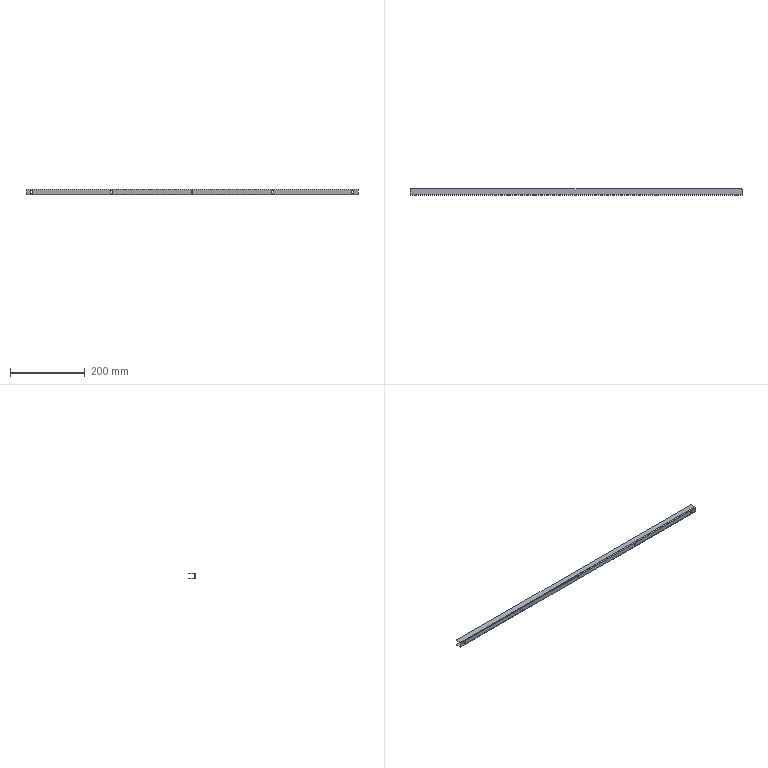Part | NX | features BREP 1 | 1 solid | 51 faces | box 890 x 17 x 15 mm | volume 40494 mm3 | plane 28 | cylinder 23 | commonest cylinder face diameters 4.8 x15 4 x6 2 x2
STEP:
#1=CARTESIAN_POINT('',(445.,14.,7.5));
#2=VERTEX_POINT('',#1);
#3=CARTESIAN_POINT('',(443.,16.,7.5));
#4=VERTEX_POINT('',#3);
#5=CARTESIAN_POINT('',(443.,14.,7.5));
#6=DIRECTION('',(0.,0.,1.));
#7=DIRECTION('',(-1.,0.,0.));
#8=AXIS2_PLACEMENT_3D('',#5,#6,#7);
#9=CIRCLE('',#8,2.);
#10=EDGE_CURVE('',#2,#4,#9,.T.);
#11=ORIENTED_EDGE('',*,*,#10,.F.);
#12=CARTESIAN_POINT('',(445.,14.,6.5));
#13=VERTEX_POINT('',#12);
#14=CARTESIAN_POINT('',(445.,14.,7.5));
#15=DIRECTION('',(0.,0.,1.));
#16=VECTOR('',#15,1000.);
#17=LINE('',#14,#16);
#18=EDGE_CURVE('',#13,#2,#17,.T.);
#19=ORIENTED_EDGE('',*,*,#18,.F.);
#20=CARTESIAN_POINT('',(443.,16.,6.5));
#21=VERTEX_POINT('',#20);
#22=CARTESIAN_POINT('',(443.,14.,6.5));
#23=DIRECTION('',(0.,0.,-1.));
#24=DIRECTION('',(-1.,0.,0.));
#25=AXIS2_PLACEMENT_3D('',#22,#23,#24);
#26=CIRCLE('',#25,2.);
#27=EDGE_CURVE('',#21,#13,#26,.T.);
#28=ORIENTED_EDGE('',*,*,#27,.F.);
#29=CARTESIAN_POINT('',(443.,16.,6.5));
#30=DIRECTION('',(0.,0.,-1.));
#31=VECTOR('',#30,1000.);
#32=LINE('',#29,#31);
#33=EDGE_CURVE('',#4,#21,#32,.T.);
#34=ORIENTED_EDGE('',*,*,#33,.F.);
#35=EDGE_LOOP('',(#11,#19,#28,#34));
#36=FACE_BOUND('',#35,.T.);
#37=CARTESIAN_POINT('',(443.,14.,7.5));
#38=DIRECTION('',(0.,0.,1.));
#39=DIRECTION('',(1.,0.,0.));
#40=AXIS2_PLACEMENT_3D('',#37,#38,#39);
#41=CYLINDRICAL_SURFACE('',#40,2.);
#42=ADVANCED_FACE('',(#36),#41,.T.);
#43=CARTESIAN_POINT('',(445.,14.,-6.5));
#44=VERTEX_POINT('',#43);
#45=CARTESIAN_POINT('',(443.,16.,-6.5));
#46=VERTEX_POINT('',#45);
#47=CARTESIAN_POINT('',(443.,14.,-6.5));
#48=DIRECTION('',(0.,0.,1.));
#49=DIRECTION('',(1.,0.,0.));
#50=AXIS2_PLACEMENT_3D('',#47,#48,#49);
#51=CIRCLE('',#50,2.);
#52=EDGE_CURVE('',#44,#46,#51,.T.);
#53=ORIENTED_EDGE('',*,*,#52,.F.);
#54=CARTESIAN_POINT('',(445.,14.,-7.5));
#55=VERTEX_POINT('',#54);
#56=CARTESIAN_POINT('',(445.,14.,-5.5));
#57=DIRECTION('',(0.,0.,1.));
#58=VECTOR('',#57,1000.);
#59=LINE('',#56,#58);
#60=EDGE_CURVE('',#55,#44,#59,.T.);
#61=ORIENTED_EDGE('',*,*,#60,.F.);
#62=CARTESIAN_POINT('',(443.,16.,-7.5));
#63=VERTEX_POINT('',#62);
#64=CARTESIAN_POINT('',(443.,14.,-7.5));
#65=DIRECTION('',(0.,0.,-1.));
#66=DIRECTION('',(1.,0.,0.));
#67=AXIS2_PLACEMENT_3D('',#64,#65,#66);
#68=CIRCLE('',#67,2.);
#69=EDGE_CURVE('',#63,#55,#68,.T.);
#70=ORIENTED_EDGE('',*,*,#69,.F.);
#71=CARTESIAN_POINT('',(443.,16.,-6.5));
#72=DIRECTION('',(0.,0.,-1.));
#73=VECTOR('',#72,1000.);
#74=LINE('',#71,#73);
#75=EDGE_CURVE('',#46,#63,#74,.T.);
#76=ORIENTED_EDGE('',*,*,#75,.F.);
#77=EDGE_LOOP('',(#53,#61,#70,#76));
#78=FACE_BOUND('',#77,.T.);
#79=CARTESIAN_POINT('',(443.,14.,-6.5));
#80=DIRECTION('',(0.,0.,-1.));
#81=DIRECTION('',(-1.,0.,0.));
#82=AXIS2_PLACEMENT_3D('',#79,#80,#81);
#83=CYLINDRICAL_SURFACE('',#82,2.);
#84=ADVANCED_FACE('',(#78),#83,.T.);
#85=CARTESIAN_POINT('',(-443.,16.,7.5));
#86=VERTEX_POINT('',#85);
#87=CARTESIAN_POINT('',(-445.,14.,7.5));
#88=VERTEX_POINT('',#87);
#89=CARTESIAN_POINT('',(-443.,14.,7.5));
#90=DIRECTION('',(0.,0.,1.));
#91=DIRECTION('',(-1.,0.,0.));
#92=AXIS2_PLACEMENT_3D('',#89,#90,#91);
#93=CIRCLE('',#92,2.);
#94=EDGE_CURVE('',#86,#88,#93,.T.);
#95=ORIENTED_EDGE('',*,*,#94,.F.);
#96=CARTESIAN_POINT('',(-443.,16.,6.5));
#97=VERTEX_POINT('',#96);
#98=CARTESIAN_POINT('',(-443.,16.,7.5));
#99=DIRECTION('',(0.,0.,1.));
#100=VECTOR('',#99,1000.);
#101=LINE('',#98,#100);
#102=EDGE_CURVE('',#97,#86,#101,.T.);
#103=ORIENTED_EDGE('',*,*,#102,.F.);
#104=CARTESIAN_POINT('',(-445.,14.,6.5));
#105=VERTEX_POINT('',#104);
#106=CARTESIAN_POINT('',(-443.,14.,6.5));
#107=DIRECTION('',(0.,0.,-1.));
#108=DIRECTION('',(-1.,0.,0.));
#109=AXIS2_PLACEMENT_3D('',#106,#107,#108);
#110=CIRCLE('',#109,2.);
#111=EDGE_CURVE('',#105,#97,#110,.T.);
#112=ORIENTED_EDGE('',*,*,#111,.F.);
#113=CARTESIAN_POINT('',(-445.,14.,5.5));
#114=DIRECTION('',(0.,0.,-1.));
#115=VECTOR('',#114,1000.);
#116=LINE('',#113,#115);
#117=EDGE_CURVE('',#88,#105,#116,.T.);
#118=ORIENTED_EDGE('',*,*,#117,.F.);
#119=EDGE_LOOP('',(#95,#103,#112,#118));
#120=FACE_BOUND('',#119,.T.);
#121=CARTESIAN_POINT('',(-443.,14.,5.5));
#122=DIRECTION('',(0.,0.,-1.));
#123=DIRECTION('',(-1.,0.,0.));
#124=AXIS2_PLACEMENT_3D('',#121,#122,#123);
#125=CYLINDRICAL_SURFACE('',#124,2.);
#126=ADVANCED_FACE('',(#120),#125,.T.);
#127=CARTESIAN_POINT('',(-443.,16.,-6.5));
#128=VERTEX_POINT('',#127);
#129=CARTESIAN_POINT('',(-445.,14.,-6.5));
#130=VERTEX_POINT('',#129);
#131=CARTESIAN_POINT('',(-443.,14.,-6.5));
#132=DIRECTION('',(0.,0.,1.));
#133=DIRECTION('',(1.,0.,0.));
#134=AXIS2_PLACEMENT_3D('',#131,#132,#133);
#135=CIRCLE('',#134,2.);
#136=EDGE_CURVE('',#128,#130,#135,.T.);
#137=ORIENTED_EDGE('',*,*,#136,.F.);
#138=CARTESIAN_POINT('',(-443.,16.,-7.5));
#139=VERTEX_POINT('',#138);
#140=CARTESIAN_POINT('',(-443.,16.,-6.5));
#141=DIRECTION('',(0.,0.,1.));
#142=VECTOR('',#141,1000.);
#143=LINE('',#140,#142);
#144=EDGE_CURVE('',#139,#128,#143,.T.);
#145=ORIENTED_EDGE('',*,*,#144,.F.);
#146=CARTESIAN_POINT('',(-445.,14.,-7.5));
#147=VERTEX_POINT('',#146);
#148=CARTESIAN_POINT('',(-443.,14.,-7.5));
#149=DIRECTION('',(0.,0.,-1.));
#150=DIRECTION('',(1.,0.,0.));
#151=AXIS2_PLACEMENT_3D('',#148,#149,#150);
#152=CIRCLE('',#151,2.);
#153=EDGE_CURVE('',#147,#139,#152,.T.);
#154=ORIENTED_EDGE('',*,*,#153,.F.);
#155=CARTESIAN_POINT('',(-445.,14.,-5.5));
#156=DIRECTION('',(0.,0.,-1.));
#157=VECTOR('',#156,1000.);
#158=LINE('',#155,#157);
#159=EDGE_CURVE('',#130,#147,#158,.T.);
#160=ORIENTED_EDGE('',*,*,#159,.F.);
#161=EDGE_LOOP('',(#137,#145,#154,#160));
#162=FACE_BOUND('',#161,.T.);
#163=CARTESIAN_POINT('',(-443.,14.,-5.5));
#164=DIRECTION('',(0.,0.,-1.));
#165=DIRECTION('',(-1.,0.,0.));
#166=AXIS2_PLACEMENT_3D('',#163,#164,#165);
#167=CYLINDRICAL_SURFACE('',#166,2.);
#168=ADVANCED_FACE('',(#162),#167,.T.);
#169=CARTESIAN_POINT('',(217.4,0.,-2.));
#170=VERTEX_POINT('',#169);
#171=CARTESIAN_POINT('',(217.4,-1.,-2.));
#172=VERTEX_POINT('',#171);
#173=CARTESIAN_POINT('',(217.4,-1.,-2.));
#174=DIRECTION('',(0.,-1.,0.));
#175=VECTOR('',#174,1000.);
#176=LINE('',#173,#175);
#177=EDGE_CURVE('',#170,#172,#176,.T.);
#178=ORIENTED_EDGE('',*,*,#177,.T.);
#179=CARTESIAN_POINT('',(217.4,-1.,2.));
#180=VERTEX_POINT('',#179);
#181=CARTESIAN_POINT('',(217.4,-1.,2.));
#182=DIRECTION('',(0.,0.,-1.));
#183=VECTOR('',#182,1000.);
#184=LINE('',#181,#183);
#185=EDGE_CURVE('',#180,#172,#184,.T.);
#186=ORIENTED_EDGE('',*,*,#185,.F.);
#187=CARTESIAN_POINT('',(217.4,0.,2.));
#188=VERTEX_POINT('',#187);
#189=CARTESIAN_POINT('',(217.4,-1.,2.));
#190=DIRECTION('',(0.,-1.,0.));
#191=VECTOR('',#190,1000.);
#192=LINE('',#189,#191);
#193=EDGE_CURVE('',#188,#180,#192,.T.);
#194=ORIENTED_EDGE('',*,*,#193,.F.);
#195=CARTESIAN_POINT('',(217.4,0.,2.));
#196=DIRECTION('',(0.,0.,-1.));
#197=VECTOR('',#196,1000.);
#198=LINE('',#195,#197);
#199=EDGE_CURVE('',#188,#170,#198,.T.);
#200=ORIENTED_EDGE('',*,*,#199,.T.);
#201=EDGE_LOOP('',(#178,#186,#194,#200));
#202=FACE_BOUND('',#201,.T.);
#203=CARTESIAN_POINT('',(217.4,-1.,2.));
#204=DIRECTION('',(1.,0.,0.));
#205=DIRECTION('',(0.,0.,-1.));
#206=AXIS2_PLACEMENT_3D('',#203,#204,#205);
#207=PLANE('',#206);
#208=ADVANCED_FACE('',(#202),#207,.F.);
#209=CARTESIAN_POINT('',(215.,-1.,4.4));
#210=VERTEX_POINT('',#209);
#211=CARTESIAN_POINT('',(215.,0.,4.4));
#212=VERTEX_POINT('',#211);
#213=CARTESIAN_POINT('',(215.,0.,4.4));
#214=DIRECTION('',(0.,1.,0.));
#215=VECTOR('',#214,1000.);
#216=LINE('',#213,#215);
#217=EDGE_CURVE('',#210,#212,#216,.T.);
#218=ORIENTED_EDGE('',*,*,#217,.F.);
#219=CARTESIAN_POINT('',(212.6,-1.,2.));
#220=VERTEX_POINT('',#219);
#221=CARTESIAN_POINT('',(215.,-1.,2.));
#222=DIRECTION('',(0.,1.,0.));
#223=DIRECTION('',(0.,0.,1.));
#224=AXIS2_PLACEMENT_3D('',#221,#222,#223);
#225=CIRCLE('',#224,2.4);
#226=EDGE_CURVE('',#220,#210,#225,.T.);
#227=ORIENTED_EDGE('',*,*,#226,.F.);
#228=CARTESIAN_POINT('',(212.6,0.,2.));
#229=VERTEX_POINT('',#228);
#230=CARTESIAN_POINT('',(212.6,0.,2.));
#231=DIRECTION('',(0.,-1.,0.));
#232=VECTOR('',#231,1000.);
#233=LINE('',#230,#232);
#234=EDGE_CURVE('',#229,#220,#233,.T.);
#235=ORIENTED_EDGE('',*,*,#234,.F.);
#236=CARTESIAN_POINT('',(215.,0.,2.));
#237=DIRECTION('',(0.,1.,0.));
#238=DIRECTION('',(0.,0.,1.));
#239=AXIS2_PLACEMENT_3D('',#236,#237,#238);
#240=CIRCLE('',#239,2.4);
#241=EDGE_CURVE('',#229,#212,#240,.T.);
#242=ORIENTED_EDGE('',*,*,#241,.T.);
#243=EDGE_LOOP('',(#218,#227,#235,#242));
#244=FACE_BOUND('',#243,.T.);
#245=CARTESIAN_POINT('',(215.,0.,2.));
#246=DIRECTION('',(0.,1.,0.));
#247=DIRECTION('',(0.,0.,1.));
#248=AXIS2_PLACEMENT_3D('',#245,#246,#247);
#249=CYLINDRICAL_SURFACE('',#248,2.4);
#250=ADVANCED_FACE('',(#244),#249,.F.);
#251=CARTESIAN_POINT('',(212.6,-1.,-2.));
#252=VERTEX_POINT('',#251);
#253=CARTESIAN_POINT('',(212.6,0.,-2.));
#254=VERTEX_POINT('',#253);
#255=CARTESIAN_POINT('',(212.6,0.,-2.));
#256=DIRECTION('',(0.,1.,0.));
#257=VECTOR('',#256,1000.);
#258=LINE('',#255,#257);
#259=EDGE_CURVE('',#252,#254,#258,.T.);
#260=ORIENTED_EDGE('',*,*,#259,.T.);
#261=CARTESIAN_POINT('',(212.6,0.,2.));
#262=DIRECTION('',(0.,0.,-1.));
#263=VECTOR('',#262,1000.);
#264=LINE('',#261,#263);
#265=EDGE_CURVE('',#229,#254,#264,.T.);
#266=ORIENTED_EDGE('',*,*,#265,.F.);
#267=ORIENTED_EDGE('',*,*,#234,.T.);
#268=CARTESIAN_POINT('',(212.6,-1.,2.));
#269=DIRECTION('',(0.,0.,-1.));
#270=VECTOR('',#269,1000.);
#271=LINE('',#268,#270);
#272=EDGE_CURVE('',#220,#252,#271,.T.);
#273=ORIENTED_EDGE('',*,*,#272,.T.);
#274=EDGE_LOOP('',(#260,#266,#267,#273));
#275=FACE_BOUND('',#274,.T.);
#276=CARTESIAN_POINT('',(212.6,0.,2.));
#277=DIRECTION('',(-1.,0.,0.));
#278=DIRECTION('',(0.,0.,1.));
#279=AXIS2_PLACEMENT_3D('',#276,#277,#278);
#280=PLANE('',#279);
#281=ADVANCED_FACE('',(#275),#280,.F.);
#282=CARTESIAN_POINT('',(215.,-1.,-2.));
#283=DIRECTION('',(0.,1.,0.));
#284=DIRECTION('',(0.,0.,1.));
#285=AXIS2_PLACEMENT_3D('',#282,#283,#284);
#286=CIRCLE('',#285,2.4);
#287=EDGE_CURVE('',#172,#252,#286,.T.);
#288=ORIENTED_EDGE('',*,*,#287,.F.);
#289=ORIENTED_EDGE('',*,*,#177,.F.);
#290=CARTESIAN_POINT('',(215.,0.,-2.));
#291=DIRECTION('',(0.,1.,0.));
#292=DIRECTION('',(0.,0.,1.));
#293=AXIS2_PLACEMENT_3D('',#290,#291,#292);
#294=CIRCLE('',#293,2.4);
#295=EDGE_CURVE('',#170,#254,#294,.T.);
#296=ORIENTED_EDGE('',*,*,#295,.T.);
#297=ORIENTED_EDGE('',*,*,#259,.F.);
#298=EDGE_LOOP('',(#288,#289,#296,#297));
#299=FACE_BOUND('',#298,.T.);
#300=CARTESIAN_POINT('',(215.,0.,-2.));
#301=DIRECTION('',(0.,1.,0.));
#302=DIRECTION('',(0.,0.,1.));
#303=AXIS2_PLACEMENT_3D('',#300,#301,#302);
#304=CYLINDRICAL_SURFACE('',#303,2.4);
#305=ADVANCED_FACE('',(#299),#304,.F.);
#306=CARTESIAN_POINT('',(432.4,0.,-2.));
#307=VERTEX_POINT('',#306);
#308=CARTESIAN_POINT('',(432.4,-1.,-2.));
#309=VERTEX_POINT('',#308);
#310=CARTESIAN_POINT('',(432.4,-1.,-2.));
#311=DIRECTION('',(0.,-1.,0.));
#312=VECTOR('',#311,1000.);
#313=LINE('',#310,#312);
#314=EDGE_CURVE('',#307,#309,#313,.T.);
#315=ORIENTED_EDGE('',*,*,#314,.T.);
#316=CARTESIAN_POINT('',(432.4,-1.,2.));
#317=VERTEX_POINT('',#316);
#318=CARTESIAN_POINT('',(432.4,-1.,2.));
#319=DIRECTION('',(0.,0.,-1.));
#320=VECTOR('',#319,1000.);
#321=LINE('',#318,#320);
#322=EDGE_CURVE('',#317,#309,#321,.T.);
#323=ORIENTED_EDGE('',*,*,#322,.F.);
#324=CARTESIAN_POINT('',(432.4,0.,2.));
#325=VERTEX_POINT('',#324);
#326=CARTESIAN_POINT('',(432.4,-1.,2.));
#327=DIRECTION('',(0.,-1.,0.));
#328=VECTOR('',#327,1000.);
#329=LINE('',#326,#328);
#330=EDGE_CURVE('',#325,#317,#329,.T.);
#331=ORIENTED_EDGE('',*,*,#330,.F.);
#332=CARTESIAN_POINT('',(432.4,0.,2.));
#333=DIRECTION('',(0.,0.,-1.));
#334=VECTOR('',#333,1000.);
#335=LINE('',#332,#334);
#336=EDGE_CURVE('',#325,#307,#335,.T.);
#337=ORIENTED_EDGE('',*,*,#336,.T.);
#338=EDGE_LOOP('',(#315,#323,#331,#337));
#339=FACE_BOUND('',#338,.T.);
#340=CARTESIAN_POINT('',(432.4,-1.,2.));
#341=DIRECTION('',(1.,0.,0.));
#342=DIRECTION('',(0.,0.,-1.));
#343=AXIS2_PLACEMENT_3D('',#340,#341,#342);
#344=PLANE('',#343);
#345=ADVANCED_FACE('',(#339),#344,.F.);
#346=CARTESIAN_POINT('',(427.6,-1.,-2.));
#347=VERTEX_POINT('',#346);
#348=CARTESIAN_POINT('',(427.6,0.,-2.));
#349=VERTEX_POINT('',#348);
#350=CARTESIAN_POINT('',(427.6,0.,-2.));
#351=DIRECTION('',(0.,1.,0.));
#352=VECTOR('',#351,1000.);
#353=LINE('',#350,#352);
#354=EDGE_CURVE('',#347,#349,#353,.T.);
#355=ORIENTED_EDGE('',*,*,#354,.T.);
#356=CARTESIAN_POINT('',(427.6,0.,2.));
#357=VERTEX_POINT('',#356);
#358=CARTESIAN_POINT('',(427.6,0.,2.));
#359=DIRECTION('',(0.,0.,-1.));
#360=VECTOR('',#359,1000.);
#361=LINE('',#358,#360);
#362=EDGE_CURVE('',#357,#349,#361,.T.);
#363=ORIENTED_EDGE('',*,*,#362,.F.);
#364=CARTESIAN_POINT('',(427.6,-1.,2.));
#365=VERTEX_POINT('',#364);
#366=CARTESIAN_POINT('',(427.6,0.,2.));
#367=DIRECTION('',(0.,-1.,0.));
#368=VECTOR('',#367,1000.);
#369=LINE('',#366,#368);
#370=EDGE_CURVE('',#357,#365,#369,.T.);
#371=ORIENTED_EDGE('',*,*,#370,.T.);
#372=CARTESIAN_POINT('',(427.6,-1.,2.));
#373=DIRECTION('',(0.,0.,-1.));
#374=VECTOR('',#373,1000.);
#375=LINE('',#372,#374);
#376=EDGE_CURVE('',#365,#347,#375,.T.);
#377=ORIENTED_EDGE('',*,*,#376,.T.);
#378=EDGE_LOOP('',(#355,#363,#371,#377));
#379=FACE_BOUND('',#378,.T.);
#380=CARTESIAN_POINT('',(427.6,0.,2.));
#381=DIRECTION('',(-1.,0.,0.));
#382=DIRECTION('',(0.,0.,1.));
#383=AXIS2_PLACEMENT_3D('',#380,#381,#382);
#384=PLANE('',#383);
#385=ADVANCED_FACE('',(#379),#384,.F.);
#386=CARTESIAN_POINT('',(430.,-1.,4.4));
#387=VERTEX_POINT('',#386);
#388=CARTESIAN_POINT('',(430.,0.,4.4));
#389=VERTEX_POINT('',#388);
#390=CARTESIAN_POINT('',(430.,0.,4.4));
#391=DIRECTION('',(0.,1.,0.));
#392=VECTOR('',#391,1000.);
#393=LINE('',#390,#392);
#394=EDGE_CURVE('',#387,#389,#393,.T.);
#395=ORIENTED_EDGE('',*,*,#394,.F.);
#396=CARTESIAN_POINT('',(430.,-1.,2.));
#397=DIRECTION('',(0.,1.,0.));
#398=DIRECTION('',(0.,0.,1.));
#399=AXIS2_PLACEMENT_3D('',#396,#397,#398);
#400=CIRCLE('',#399,2.4);
#401=EDGE_CURVE('',#365,#387,#400,.T.);
#402=ORIENTED_EDGE('',*,*,#401,.F.);
#403=ORIENTED_EDGE('',*,*,#370,.F.);
#404=CARTESIAN_POINT('',(430.,0.,2.));
#405=DIRECTION('',(0.,1.,0.));
#406=DIRECTION('',(0.,0.,1.));
#407=AXIS2_PLACEMENT_3D('',#404,#405,#406);
#408=CIRCLE('',#407,2.4);
#409=EDGE_CURVE('',#357,#389,#408,.T.);
#410=ORIENTED_EDGE('',*,*,#409,.T.);
#411=EDGE_LOOP('',(#395,#402,#403,#410));
#412=FACE_BOUND('',#411,.T.);
#413=CARTESIAN_POINT('',(430.,0.,2.));
#414=DIRECTION('',(0.,1.,0.));
#415=DIRECTION('',(0.,0.,1.));
#416=AXIS2_PLACEMENT_3D('',#413,#414,#415);
#417=CYLINDRICAL_SURFACE('',#416,2.4);
#418=ADVANCED_FACE('',(#412),#417,.F.);
#419=CARTESIAN_POINT('',(430.,-1.,-2.));
#420=DIRECTION('',(0.,1.,0.));
#421=DIRECTION('',(0.,0.,1.));
#422=AXIS2_PLACEMENT_3D('',#419,#420,#421);
#423=CIRCLE('',#422,2.4);
#424=EDGE_CURVE('',#309,#347,#423,.T.);
#425=ORIENTED_EDGE('',*,*,#424,.F.);
#426=ORIENTED_EDGE('',*,*,#314,.F.);
#427=CARTESIAN_POINT('',(430.,0.,-2.));
#428=DIRECTION('',(0.,1.,0.));
#429=DIRECTION('',(0.,0.,1.));
#430=AXIS2_PLACEMENT_3D('',#427,#428,#429);
#431=CIRCLE('',#430,2.4);
#432=EDGE_CURVE('',#307,#349,#431,.T.);
#433=ORIENTED_EDGE('',*,*,#432,.T.);
#434=ORIENTED_EDGE('',*,*,#354,.F.);
#435=EDGE_LOOP('',(#425,#426,#433,#434));
#436=FACE_BOUND('',#435,.T.);
#437=CARTESIAN_POINT('',(430.,0.,-2.));
#438=DIRECTION('',(0.,1.,0.));
#439=DIRECTION('',(0.,0.,1.));
#440=AXIS2_PLACEMENT_3D('',#437,#438,#439);
#441=CYLINDRICAL_SURFACE('',#440,2.4);
#442=ADVANCED_FACE('',(#436),#441,.F.);
#443=CARTESIAN_POINT('',(-445.,1.,-6.5));
#444=VERTEX_POINT('',#443);
#445=CARTESIAN_POINT('',(-445.,0.,-6.5));
#446=DIRECTION('',(0.,1.,0.));
#447=VECTOR('',#446,1000.);
#448=LINE('',#445,#447);
#449=EDGE_CURVE('',#444,#130,#448,.T.);
#450=ORIENTED_EDGE('',*,*,#449,.T.);
#451=ORIENTED_EDGE('',*,*,#159,.T.);
#452=CARTESIAN_POINT('',(-445.,1.,-7.5));
#453=VERTEX_POINT('',#452);
#454=CARTESIAN_POINT('',(-445.,0.,-7.5));
#455=DIRECTION('',(0.,1.,0.));
#456=VECTOR('',#455,1000.);
#457=LINE('',#454,#456);
#458=EDGE_CURVE('',#453,#147,#457,.T.);
#459=ORIENTED_EDGE('',*,*,#458,.F.);
#460=CARTESIAN_POINT('',(-445.,1.,-7.5));
#461=DIRECTION('',(0.,0.,1.));
#462=VECTOR('',#461,1000.);
#463=LINE('',#460,#462);
#464=EDGE_CURVE('',#453,#444,#463,.T.);
#465=ORIENTED_EDGE('',*,*,#464,.T.);
#466=EDGE_LOOP('',(#450,#451,#459,#465));
#467=FACE_BOUND('',#466,.T.);
#468=CARTESIAN_POINT('',(-445.,1.,-5.5));
#469=DIRECTION('',(-1.,0.,0.));
#470=DIRECTION('',(0.,0.,1.));
#471=AXIS2_PLACEMENT_3D('',#468,#469,#470);
#472=PLANE('',#471);
#473=ADVANCED_FACE('',(#467),#472,.T.);
#474=CARTESIAN_POINT('',(445.,1.,6.5));
#475=VERTEX_POINT('',#474);
#476=CARTESIAN_POINT('',(445.,0.,6.5));
#477=DIRECTION('',(0.,-1.,0.));
#478=VECTOR('',#477,1000.);
#479=LINE('',#476,#478);
#480=EDGE_CURVE('',#13,#475,#479,.T.);
#481=ORIENTED_EDGE('',*,*,#480,.F.);
#482=ORIENTED_EDGE('',*,*,#18,.T.);
#483=CARTESIAN_POINT('',(445.,1.,7.5));
#484=VERTEX_POINT('',#483);
#485=CARTESIAN_POINT('',(445.,0.,7.5));
#486=DIRECTION('',(0.,-1.,0.));
#487=VECTOR('',#486,1000.);
#488=LINE('',#485,#487);
#489=EDGE_CURVE('',#2,#484,#488,.T.);
#490=ORIENTED_EDGE('',*,*,#489,.T.);
#491=CARTESIAN_POINT('',(445.,1.,7.5));
#492=DIRECTION('',(0.,0.,-1.));
#493=VECTOR('',#492,1000.);
#494=LINE('',#491,#493);
#495=EDGE_CURVE('',#484,#475,#494,.T.);
#496=ORIENTED_EDGE('',*,*,#495,.T.);
#497=EDGE_LOOP('',(#481,#482,#490,#496));
#498=FACE_BOUND('',#497,.T.);
#499=CARTESIAN_POINT('',(445.,1.,-5.5));
#500=DIRECTION('',(-1.,0.,0.));
#501=DIRECTION('',(0.,0.,1.));
#502=AXIS2_PLACEMENT_3D('',#499,#500,#501);
#503=PLANE('',#502);
#504=ADVANCED_FACE('',(#498),#503,.F.);
#505=CARTESIAN_POINT('',(-445.,-1.,-5.5));
#506=VERTEX_POINT('',#505);
#507=CARTESIAN_POINT('',(-445.,1.,-5.5));
#508=DIRECTION('',(1.,0.,0.));
#509=DIRECTION('',(0.,0.,-1.));
#510=AXIS2_PLACEMENT_3D('',#507,#508,#509);
#511=CIRCLE('',#510,2.);
#512=EDGE_CURVE('',#506,#453,#511,.T.);
#513=ORIENTED_EDGE('',*,*,#512,.T.);
#514=CARTESIAN_POINT('',(445.,1.,-7.5));
#515=VERTEX_POINT('',#514);
#516=CARTESIAN_POINT('',(445.,1.,-7.5));
#517=DIRECTION('',(-1.,0.,0.));
#518=VECTOR('',#517,1000.);
#519=LINE('',#516,#518);
#520=EDGE_CURVE('',#515,#453,#519,.T.);
#521=ORIENTED_EDGE('',*,*,#520,.F.);
#522=CARTESIAN_POINT('',(445.,-1.,-5.5));
#523=VERTEX_POINT('',#522);
#524=CARTESIAN_POINT('',(445.,1.,-5.5));
#525=DIRECTION('',(1.,0.,0.));
#526=DIRECTION('',(0.,0.,-1.));
#527=AXIS2_PLACEMENT_3D('',#524,#525,#526);
#528=CIRCLE('',#527,2.);
#529=EDGE_CURVE('',#523,#515,#528,.T.);
#530=ORIENTED_EDGE('',*,*,#529,.F.);
#531=CARTESIAN_POINT('',(445.,-1.,-5.5));
#532=DIRECTION('',(-1.,0.,0.));
#533=VECTOR('',#532,1000.);
#534=LINE('',#531,#533);
#535=EDGE_CURVE('',#523,#506,#534,.T.);
#536=ORIENTED_EDGE('',*,*,#535,.T.);
#537=EDGE_LOOP('',(#513,#521,#530,#536));
#538=FACE_BOUND('',#537,.T.);
#539=CARTESIAN_POINT('',(445.,1.,-5.5));
#540=DIRECTION('',(-1.,0.,0.));
#541=DIRECTION('',(0.,0.,1.));
#542=AXIS2_PLACEMENT_3D('',#539,#540,#541);
#543=CYLINDRICAL_SURFACE('',#542,2.);
#544=ADVANCED_FACE('',(#538),#543,.T.);
#545=CARTESIAN_POINT('',(-427.6,-1.,-2.));
#546=VERTEX_POINT('',#545);
#547=CARTESIAN_POINT('',(-432.4,-1.,-2.));
#548=VERTEX_POINT('',#547);
#549=CARTESIAN_POINT('',(-430.,-1.,-2.));
#550=DIRECTION('',(0.,1.,0.));
#551=DIRECTION('',(0.,0.,1.));
#552=AXIS2_PLACEMENT_3D('',#549,#550,#551);
#553=CIRCLE('',#552,2.4);
#554=EDGE_CURVE('',#546,#548,#553,.T.);
#555=ORIENTED_EDGE('',*,*,#554,.T.);
#556=CARTESIAN_POINT('',(-432.4,-1.,2.));
#557=VERTEX_POINT('',#556);
#558=CARTESIAN_POINT('',(-432.4,-1.,2.));
#559=DIRECTION('',(0.,0.,-1.));
#560=VECTOR('',#559,1000.);
#561=LINE('',#558,#560);
#562=EDGE_CURVE('',#557,#548,#561,.T.);
#563=ORIENTED_EDGE('',*,*,#562,.F.);
#564=CARTESIAN_POINT('',(-430.,-1.,4.4));
#565=VERTEX_POINT('',#564);
#566=CARTESIAN_POINT('',(-430.,-1.,2.));
#567=DIRECTION('',(0.,1.,0.));
#568=DIRECTION('',(0.,0.,1.));
#569=AXIS2_PLACEMENT_3D('',#566,#567,#568);
#570=CIRCLE('',#569,2.4);
#571=EDGE_CURVE('',#557,#565,#570,.T.);
#572=ORIENTED_EDGE('',*,*,#571,.T.);
#573=CARTESIAN_POINT('',(-427.6,-1.,2.));
#574=VERTEX_POINT('',#573);
#575=CARTESIAN_POINT('',(-430.,-1.,2.));
#576=DIRECTION('',(0.,1.,0.));
#577=DIRECTION('',(0.,0.,1.));
#578=AXIS2_PLACEMENT_3D('',#575,#576,#577);
#579=CIRCLE('',#578,2.4);
#580=EDGE_CURVE('',#565,#574,#579,.T.);
#581=ORIENTED_EDGE('',*,*,#580,.T.);
#582=CARTESIAN_POINT('',(-427.6,-1.,2.));
#583=DIRECTION('',(0.,0.,-1.));
#584=VECTOR('',#583,1000.);
#585=LINE('',#582,#584);
#586=EDGE_CURVE('',#574,#546,#585,.T.);
#587=ORIENTED_EDGE('',*,*,#586,.T.);
#588=EDGE_LOOP('',(#555,#563,#572,#581,#587));
#589=FACE_BOUND('',#588,.T.);
#590=CARTESIAN_POINT('',(-212.6,-1.,-2.));
#591=VERTEX_POINT('',#590);
#592=CARTESIAN_POINT('',(-217.4,-1.,-2.));
#593=VERTEX_POINT('',#592);
#594=CARTESIAN_POINT('',(-215.,-1.,-2.));
#595=DIRECTION('',(0.,1.,0.));
#596=DIRECTION('',(0.,0.,1.));
#597=AXIS2_PLACEMENT_3D('',#594,#595,#596);
#598=CIRCLE('',#597,2.4);
#599=EDGE_CURVE('',#591,#593,#598,.T.);
#600=ORIENTED_EDGE('',*,*,#599,.T.);
#601=CARTESIAN_POINT('',(-217.4,-1.,2.));
#602=VERTEX_POINT('',#601);
#603=CARTESIAN_POINT('',(-217.4,-1.,2.));
#604=DIRECTION('',(0.,0.,-1.));
#605=VECTOR('',#604,1000.);
#606=LINE('',#603,#605);
#607=EDGE_CURVE('',#602,#593,#606,.T.);
#608=ORIENTED_EDGE('',*,*,#607,.F.);
#609=CARTESIAN_POINT('',(-215.,-1.,4.4));
#610=VERTEX_POINT('',#609);
#611=CARTESIAN_POINT('',(-215.,-1.,2.));
#612=DIRECTION('',(0.,1.,0.));
#613=DIRECTION('',(0.,0.,1.));
#614=AXIS2_PLACEMENT_3D('',#611,#612,#613);
#615=CIRCLE('',#614,2.4);
#616=EDGE_CURVE('',#602,#610,#615,.T.);
#617=ORIENTED_EDGE('',*,*,#616,.T.);
#618=CARTESIAN_POINT('',(-212.6,-1.,2.));
#619=VERTEX_POINT('',#618);
#620=CARTESIAN_POINT('',(-215.,-1.,2.));
#621=DIRECTION('',(0.,1.,0.));
#622=DIRECTION('',(0.,0.,1.));
#623=AXIS2_PLACEMENT_3D('',#620,#621,#622);
#624=CIRCLE('',#623,2.4);
#625=EDGE_CURVE('',#610,#619,#624,.T.);
#626=ORIENTED_EDGE('',*,*,#625,.T.);
#627=CARTESIAN_POINT('',(-212.6,-1.,2.));
#628=DIRECTION('',(0.,0.,-1.));
#629=VECTOR('',#628,1000.);
#630=LINE('',#627,#629);
#631=EDGE_CURVE('',#619,#591,#630,.T.);
#632=ORIENTED_EDGE('',*,*,#631,.T.);
#633=EDGE_LOOP('',(#600,#608,#617,#626,#632));
#634=FACE_BOUND('',#633,.T.);
#635=CARTESIAN_POINT('',(2.4,-1.,-2.));
#636=VERTEX_POINT('',#635);
#637=CARTESIAN_POINT('',(-2.4,-1.,-2.));
#638=VERTEX_POINT('',#637);
#639=CARTESIAN_POINT('',(0.,-1.,-2.));
#640=DIRECTION('',(0.,1.,0.));
#641=DIRECTION('',(0.,0.,1.));
#642=AXIS2_PLACEMENT_3D('',#639,#640,#641);
#643=CIRCLE('',#642,2.4);
#644=EDGE_CURVE('',#636,#638,#643,.T.);
#645=ORIENTED_EDGE('',*,*,#644,.T.);
#646=CARTESIAN_POINT('',(-2.4,-1.,2.));
#647=VERTEX_POINT('',#646);
#648=CARTESIAN_POINT('',(-2.4,-1.,2.));
#649=DIRECTION('',(0.,0.,-1.));
#650=VECTOR('',#649,1000.);
#651=LINE('',#648,#650);
#652=EDGE_CURVE('',#647,#638,#651,.T.);
#653=ORIENTED_EDGE('',*,*,#652,.F.);
#654=CARTESIAN_POINT('',(0.,-1.,4.4));
#655=VERTEX_POINT('',#654);
#656=CARTESIAN_POINT('',(0.,-1.,2.));
#657=DIRECTION('',(0.,1.,0.));
#658=DIRECTION('',(0.,0.,1.));
#659=AXIS2_PLACEMENT_3D('',#656,#657,#658);
#660=CIRCLE('',#659,2.4);
#661=EDGE_CURVE('',#647,#655,#660,.T.);
#662=ORIENTED_EDGE('',*,*,#661,.T.);
#663=CARTESIAN_POINT('',(2.4,-1.,2.));
#664=VERTEX_POINT('',#663);
#665=CARTESIAN_POINT('',(0.,-1.,2.));
#666=DIRECTION('',(0.,1.,0.));
#667=DIRECTION('',(0.,0.,1.));
#668=AXIS2_PLACEMENT_3D('',#665,#666,#667);
#669=CIRCLE('',#668,2.4);
#670=EDGE_CURVE('',#655,#664,#669,.T.);
#671=ORIENTED_EDGE('',*,*,#670,.T.);
#672=CARTESIAN_POINT('',(2.4,-1.,2.));
#673=DIRECTION('',(0.,0.,-1.));
#674=VECTOR('',#673,1000.);
#675=LINE('',#672,#674);
#676=EDGE_CURVE('',#664,#636,#675,.T.);
#677=ORIENTED_EDGE('',*,*,#676,.T.);
#678=EDGE_LOOP('',(#645,#653,#662,#671,#677));
#679=FACE_BOUND('',#678,.T.);
#680=CARTESIAN_POINT('',(-445.,-1.,5.5));
#681=VERTEX_POINT('',#680);
#682=CARTESIAN_POINT('',(-445.,-1.,6.5));
#683=DIRECTION('',(0.,0.,-1.));
#684=VECTOR('',#683,1000.);
#685=LINE('',#682,#684);
#686=EDGE_CURVE('',#681,#506,#685,.T.);
#687=ORIENTED_EDGE('',*,*,#686,.T.);
#688=ORIENTED_EDGE('',*,*,#535,.F.);
#689=CARTESIAN_POINT('',(445.,-1.,5.5));
#690=VERTEX_POINT('',#689);
#691=CARTESIAN_POINT('',(445.,-1.,6.5));
#692=DIRECTION('',(0.,0.,-1.));
#693=VECTOR('',#692,1000.);
#694=LINE('',#691,#693);
#695=EDGE_CURVE('',#690,#523,#694,.T.);
#696=ORIENTED_EDGE('',*,*,#695,.F.);
#697=CARTESIAN_POINT('',(445.,-1.,5.5));
#698=DIRECTION('',(-1.,0.,0.));
#699=VECTOR('',#698,1000.);
#700=LINE('',#697,#699);
#701=EDGE_CURVE('',#690,#681,#700,.T.);
#702=ORIENTED_EDGE('',*,*,#701,.T.);
#703=EDGE_LOOP('',(#687,#688,#696,#702));
#704=FACE_BOUND('',#703,.T.);
#705=ORIENTED_EDGE('',*,*,#322,.T.);
#706=ORIENTED_EDGE('',*,*,#424,.T.);
#707=ORIENTED_EDGE('',*,*,#376,.F.);
#708=ORIENTED_EDGE('',*,*,#401,.T.);
#709=CARTESIAN_POINT('',(430.,-1.,2.));
#710=DIRECTION('',(0.,1.,0.));
#711=DIRECTION('',(0.,0.,1.));
#712=AXIS2_PLACEMENT_3D('',#709,#710,#711);
#713=CIRCLE('',#712,2.4);
#714=EDGE_CURVE('',#387,#317,#713,.T.);
#715=ORIENTED_EDGE('',*,*,#714,.T.);
#716=EDGE_LOOP('',(#705,#706,#707,#708,#715));
#717=FACE_BOUND('',#716,.T.);
#718=ORIENTED_EDGE('',*,*,#185,.T.);
#719=ORIENTED_EDGE('',*,*,#287,.T.);
#720=ORIENTED_EDGE('',*,*,#272,.F.);
#721=ORIENTED_EDGE('',*,*,#226,.T.);
#722=CARTESIAN_POINT('',(215.,-1.,2.));
#723=DIRECTION('',(0.,1.,0.));
#724=DIRECTION('',(0.,0.,1.));
#725=AXIS2_PLACEMENT_3D('',#722,#723,#724);
#726=CIRCLE('',#725,2.4);
#727=EDGE_CURVE('',#210,#180,#726,.T.);
#728=ORIENTED_EDGE('',*,*,#727,.T.);
#729=EDGE_LOOP('',(#718,#719,#720,#721,#728));
#730=FACE_BOUND('',#729,.T.);
#731=CARTESIAN_POINT('',(445.,-1.,6.5));
#732=DIRECTION('',(0.,1.,0.));
#733=DIRECTION('',(0.,0.,1.));
#734=AXIS2_PLACEMENT_3D('',#731,#732,#733);
#735=PLANE('',#734);
#736=ADVANCED_FACE('',(#589,#634,#679,#704,#717,#730),#735,.F.);
#737=CARTESIAN_POINT('',(-445.,1.,7.5));
#738=VERTEX_POINT('',#737);
#739=CARTESIAN_POINT('',(-445.,1.,5.5));
#740=DIRECTION('',(1.,0.,0.));
#741=DIRECTION('',(0.,0.,-1.));
#742=AXIS2_PLACEMENT_3D('',#739,#740,#741);
#743=CIRCLE('',#742,2.);
#744=EDGE_CURVE('',#738,#681,#743,.T.);
#745=ORIENTED_EDGE('',*,*,#744,.T.);
#746=ORIENTED_EDGE('',*,*,#701,.F.);
#747=CARTESIAN_POINT('',(445.,1.,5.5));
#748=DIRECTION('',(1.,0.,0.));
#749=DIRECTION('',(0.,0.,-1.));
#750=AXIS2_PLACEMENT_3D('',#747,#748,#749);
#751=CIRCLE('',#750,2.);
#752=EDGE_CURVE('',#484,#690,#751,.T.);
#753=ORIENTED_EDGE('',*,*,#752,.F.);
#754=CARTESIAN_POINT('',(445.,1.,7.5));
#755=DIRECTION('',(-1.,0.,0.));
#756=VECTOR('',#755,1000.);
#757=LINE('',#754,#756);
#758=EDGE_CURVE('',#484,#738,#757,.T.);
#759=ORIENTED_EDGE('',*,*,#758,.T.);
#760=EDGE_LOOP('',(#745,#746,#753,#759));
#761=FACE_BOUND('',#760,.T.);
#762=CARTESIAN_POINT('',(445.,1.,5.5));
#763=DIRECTION('',(-1.,0.,0.));
#764=DIRECTION('',(0.,0.,1.));
#765=AXIS2_PLACEMENT_3D('',#762,#763,#764);
#766=CYLINDRICAL_SURFACE('',#765,2.);
#767=ADVANCED_FACE('',(#761),#766,.T.);
#768=CARTESIAN_POINT('',(445.,16.,7.5));
#769=DIRECTION('',(-1.,0.,0.));
#770=VECTOR('',#769,1000.);
#771=LINE('',#768,#770);
#772=EDGE_CURVE('',#4,#86,#771,.T.);
#773=ORIENTED_EDGE('',*,*,#772,.T.);
#774=ORIENTED_EDGE('',*,*,#94,.T.);
#775=CARTESIAN_POINT('',(-445.,0.,7.5));
#776=DIRECTION('',(0.,-1.,0.));
#777=VECTOR('',#776,1000.);
#778=LINE('',#775,#777);
#779=EDGE_CURVE('',#88,#738,#778,.T.);
#780=ORIENTED_EDGE('',*,*,#779,.T.);
#781=ORIENTED_EDGE('',*,*,#758,.F.);
#782=ORIENTED_EDGE('',*,*,#489,.F.);
#783=ORIENTED_EDGE('',*,*,#10,.T.);
#784=EDGE_LOOP('',(#773,#774,#780,#781,#782,#783));
#785=FACE_BOUND('',#784,.T.);
#786=CARTESIAN_POINT('',(445.,0.,7.5));
#787=DIRECTION('',(0.,0.,-1.));
#788=DIRECTION('',(-1.,0.,0.));
#789=AXIS2_PLACEMENT_3D('',#786,#787,#788);
#790=PLANE('',#789);
#791=ADVANCED_FACE('',(#785),#790,.F.);
#792=CARTESIAN_POINT('',(445.,16.,6.5));
#793=DIRECTION('',(-1.,0.,0.));
#794=VECTOR('',#793,1000.);
#795=LINE('',#792,#794);
#796=EDGE_CURVE('',#21,#97,#795,.T.);
#797=ORIENTED_EDGE('',*,*,#796,.T.);
#798=ORIENTED_EDGE('',*,*,#102,.T.);
#799=ORIENTED_EDGE('',*,*,#772,.F.);
#800=ORIENTED_EDGE('',*,*,#33,.T.);
#801=EDGE_LOOP('',(#797,#798,#799,#800));
#802=FACE_BOUND('',#801,.T.);
#803=CARTESIAN_POINT('',(445.,16.,7.5));
#804=DIRECTION('',(0.,1.,0.));
#805=DIRECTION('',(0.,0.,1.));
#806=AXIS2_PLACEMENT_3D('',#803,#804,#805);
#807=PLANE('',#806);
#808=ADVANCED_FACE('',(#802),#807,.T.);
#809=CARTESIAN_POINT('',(-445.,1.,6.5));
#810=VERTEX_POINT('',#809);
#811=CARTESIAN_POINT('',(-445.,0.,6.5));
#812=DIRECTION('',(0.,-1.,0.));
#813=VECTOR('',#812,1000.);
#814=LINE('',#811,#813);
#815=EDGE_CURVE('',#105,#810,#814,.T.);
#816=ORIENTED_EDGE('',*,*,#815,.F.);
#817=ORIENTED_EDGE('',*,*,#111,.T.);
#818=ORIENTED_EDGE('',*,*,#796,.F.);
#819=ORIENTED_EDGE('',*,*,#27,.T.);
#820=ORIENTED_EDGE('',*,*,#480,.T.);
#821=CARTESIAN_POINT('',(445.,1.,6.5));
#822=DIRECTION('',(-1.,0.,0.));
#823=VECTOR('',#822,1000.);
#824=LINE('',#821,#823);
#825=EDGE_CURVE('',#475,#810,#824,.T.);
#826=ORIENTED_EDGE('',*,*,#825,.T.);
#827=EDGE_LOOP('',(#816,#817,#818,#819,#820,#826));
#828=FACE_BOUND('',#827,.T.);
#829=CARTESIAN_POINT('',(445.,0.,6.5));
#830=DIRECTION('',(0.,0.,-1.));
#831=DIRECTION('',(-1.,0.,0.));
#832=AXIS2_PLACEMENT_3D('',#829,#830,#831);
#833=PLANE('',#832);
#834=ADVANCED_FACE('',(#828),#833,.T.);
#835=CARTESIAN_POINT('',(-445.,0.,5.5));
#836=VERTEX_POINT('',#835);
#837=CARTESIAN_POINT('',(-445.,1.,5.5));
#838=DIRECTION('',(1.,0.,0.));
#839=DIRECTION('',(0.,0.,1.));
#840=AXIS2_PLACEMENT_3D('',#837,#838,#839);
#841=CIRCLE('',#840,1.);
#842=EDGE_CURVE('',#810,#836,#841,.T.);
#843=ORIENTED_EDGE('',*,*,#842,.F.);
#844=ORIENTED_EDGE('',*,*,#825,.F.);
#845=CARTESIAN_POINT('',(445.,0.,5.5));
#846=VERTEX_POINT('',#845);
#847=CARTESIAN_POINT('',(445.,1.,5.5));
#848=DIRECTION('',(1.,0.,0.));
#849=DIRECTION('',(0.,0.,1.));
#850=AXIS2_PLACEMENT_3D('',#847,#848,#849);
#851=CIRCLE('',#850,1.);
#852=EDGE_CURVE('',#475,#846,#851,.T.);
#853=ORIENTED_EDGE('',*,*,#852,.T.);
#854=CARTESIAN_POINT('',(445.,0.,5.5));
#855=DIRECTION('',(-1.,0.,0.));
#856=VECTOR('',#855,1000.);
#857=LINE('',#854,#856);
#858=EDGE_CURVE('',#846,#836,#857,.T.);
#859=ORIENTED_EDGE('',*,*,#858,.T.);
#860=EDGE_LOOP('',(#843,#844,#853,#859));
#861=FACE_BOUND('',#860,.T.);
#862=CARTESIAN_POINT('',(445.,1.,5.5));
#863=DIRECTION('',(-1.,0.,0.));
#864=DIRECTION('',(0.,0.,1.));
#865=AXIS2_PLACEMENT_3D('',#862,#863,#864);
#866=CYLINDRICAL_SURFACE('',#865,1.);
#867=ADVANCED_FACE('',(#861),#866,.F.);
#868=CARTESIAN_POINT('',(-445.,0.,-5.5));
#869=VERTEX_POINT('',#868);
#870=CARTESIAN_POINT('',(-445.,1.,-5.5));
#871=DIRECTION('',(1.,0.,0.));
#872=DIRECTION('',(0.,0.,1.));
#873=AXIS2_PLACEMENT_3D('',#870,#871,#872);
#874=CIRCLE('',#873,1.);
#875=EDGE_CURVE('',#869,#444,#874,.T.);
#876=ORIENTED_EDGE('',*,*,#875,.F.);
#877=CARTESIAN_POINT('',(445.,0.,-5.5));
#878=VERTEX_POINT('',#877);
#879=CARTESIAN_POINT('',(445.,0.,-5.5));
#880=DIRECTION('',(-1.,0.,0.));
#881=VECTOR('',#880,1000.);
#882=LINE('',#879,#881);
#883=EDGE_CURVE('',#878,#869,#882,.T.);
#884=ORIENTED_EDGE('',*,*,#883,.F.);
#885=CARTESIAN_POINT('',(445.,1.,-6.5));
#886=VERTEX_POINT('',#885);
#887=CARTESIAN_POINT('',(445.,1.,-5.5));
#888=DIRECTION('',(1.,0.,0.));
#889=DIRECTION('',(0.,0.,1.));
#890=AXIS2_PLACEMENT_3D('',#887,#888,#889);
#891=CIRCLE('',#890,1.);
#892=EDGE_CURVE('',#878,#886,#891,.T.);
#893=ORIENTED_EDGE('',*,*,#892,.T.);
#894=CARTESIAN_POINT('',(445.,1.,-6.5));
#895=DIRECTION('',(-1.,0.,0.));
#896=VECTOR('',#895,1000.);
#897=LINE('',#894,#896);
#898=EDGE_CURVE('',#886,#444,#897,.T.);
#899=ORIENTED_EDGE('',*,*,#898,.T.);
#900=EDGE_LOOP('',(#876,#884,#893,#899));
#901=FACE_BOUND('',#900,.T.);
#902=CARTESIAN_POINT('',(445.,1.,-5.5));
#903=DIRECTION('',(-1.,0.,0.));
#904=DIRECTION('',(0.,0.,1.));
#905=AXIS2_PLACEMENT_3D('',#902,#903,#904);
#906=CYLINDRICAL_SURFACE('',#905,1.);
#907=ADVANCED_FACE('',(#901),#906,.F.);
#908=CARTESIAN_POINT('',(445.,16.,-6.5));
#909=DIRECTION('',(-1.,0.,0.));
#910=VECTOR('',#909,1000.);
#911=LINE('',#908,#910);
#912=EDGE_CURVE('',#46,#128,#911,.T.);
#913=ORIENTED_EDGE('',*,*,#912,.T.);
#914=ORIENTED_EDGE('',*,*,#136,.T.);
#915=ORIENTED_EDGE('',*,*,#449,.F.);
#916=ORIENTED_EDGE('',*,*,#898,.F.);
#917=CARTESIAN_POINT('',(445.,0.,-6.5));
#918=DIRECTION('',(0.,1.,0.));
#919=VECTOR('',#918,1000.);
#920=LINE('',#917,#919);
#921=EDGE_CURVE('',#886,#44,#920,.T.);
#922=ORIENTED_EDGE('',*,*,#921,.T.);
#923=ORIENTED_EDGE('',*,*,#52,.T.);
#924=EDGE_LOOP('',(#913,#914,#915,#916,#922,#923));
#925=FACE_BOUND('',#924,.T.);
#926=CARTESIAN_POINT('',(445.,0.,-6.5));
#927=DIRECTION('',(0.,0.,1.));
#928=DIRECTION('',(1.,0.,0.));
#929=AXIS2_PLACEMENT_3D('',#926,#927,#928);
#930=PLANE('',#929);
#931=ADVANCED_FACE('',(#925),#930,.T.);
#932=CARTESIAN_POINT('',(445.,16.,-7.5));
#933=DIRECTION('',(-1.,0.,0.));
#934=VECTOR('',#933,1000.);
#935=LINE('',#932,#934);
#936=EDGE_CURVE('',#63,#139,#935,.T.);
#937=ORIENTED_EDGE('',*,*,#936,.T.);
#938=ORIENTED_EDGE('',*,*,#144,.T.);
#939=ORIENTED_EDGE('',*,*,#912,.F.);
#940=ORIENTED_EDGE('',*,*,#75,.T.);
#941=EDGE_LOOP('',(#937,#938,#939,#940));
#942=FACE_BOUND('',#941,.T.);
#943=CARTESIAN_POINT('',(445.,16.,-6.5));
#944=DIRECTION('',(0.,1.,0.));
#945=DIRECTION('',(0.,0.,1.));
#946=AXIS2_PLACEMENT_3D('',#943,#944,#945);
#947=PLANE('',#946);
#948=ADVANCED_FACE('',(#942),#947,.T.);
#949=ORIENTED_EDGE('',*,*,#458,.T.);
#950=ORIENTED_EDGE('',*,*,#153,.T.);
#951=ORIENTED_EDGE('',*,*,#936,.F.);
#952=ORIENTED_EDGE('',*,*,#69,.T.);
#953=CARTESIAN_POINT('',(445.,0.,-7.5));
#954=DIRECTION('',(0.,1.,0.));
#955=VECTOR('',#954,1000.);
#956=LINE('',#953,#955);
#957=EDGE_CURVE('',#515,#55,#956,.T.);
#958=ORIENTED_EDGE('',*,*,#957,.F.);
#959=ORIENTED_EDGE('',*,*,#520,.T.);
#960=EDGE_LOOP('',(#949,#950,#951,#952,#958,#959));
#961=FACE_BOUND('',#960,.T.);
#962=CARTESIAN_POINT('',(445.,0.,-7.5));
#963=DIRECTION('',(0.,0.,1.));
#964=DIRECTION('',(1.,0.,0.));
#965=AXIS2_PLACEMENT_3D('',#962,#963,#964);
#966=PLANE('',#965);
#967=ADVANCED_FACE('',(#961),#966,.F.);
#968=CARTESIAN_POINT('',(-445.,0.,6.5));
#969=DIRECTION('',(0.,0.,-1.));
#970=VECTOR('',#969,1000.);
#971=LINE('',#968,#970);
#972=EDGE_CURVE('',#836,#869,#971,.T.);
#973=ORIENTED_EDGE('',*,*,#972,.T.);
#974=CARTESIAN_POINT('',(-445.,0.,-5.5));
#975=DIRECTION('',(0.,-1.,0.));
#976=VECTOR('',#975,1000.);
#977=LINE('',#974,#976);
#978=EDGE_CURVE('',#869,#506,#977,.T.);
#979=ORIENTED_EDGE('',*,*,#978,.T.);
#980=ORIENTED_EDGE('',*,*,#686,.F.);
#981=CARTESIAN_POINT('',(-445.,-1.,5.5));
#982=DIRECTION('',(0.,1.,0.));
#983=VECTOR('',#982,1000.);
#984=LINE('',#981,#983);
#985=EDGE_CURVE('',#681,#836,#984,.T.);
#986=ORIENTED_EDGE('',*,*,#985,.T.);
#987=EDGE_LOOP('',(#973,#979,#980,#986));
#988=FACE_BOUND('',#987,.T.);
#989=CARTESIAN_POINT('',(-445.,1.,-7.5));
#990=DIRECTION('',(-1.,0.,0.));
#991=DIRECTION('',(0.,0.,1.));
#992=AXIS2_PLACEMENT_3D('',#989,#990,#991);
#993=PLANE('',#992);
#994=ADVANCED_FACE('',(#988),#993,.T.);
#995=ORIENTED_EDGE('',*,*,#978,.F.);
#996=ORIENTED_EDGE('',*,*,#875,.T.);
#997=ORIENTED_EDGE('',*,*,#464,.F.);
#998=ORIENTED_EDGE('',*,*,#512,.F.);
#999=EDGE_LOOP('',(#995,#996,#997,#998));
#1000=FACE_BOUND('',#999,.T.);
#1001=CARTESIAN_POINT('',(-445.,0.,-5.5));
#1002=DIRECTION('',(-1.,0.,0.));
#1003=DIRECTION('',(0.,0.,1.));
#1004=AXIS2_PLACEMENT_3D('',#1001,#1002,#1003);
#1005=PLANE('',#1004);
#1006=ADVANCED_FACE('',(#1000),#1005,.T.);
#1007=ORIENTED_EDGE('',*,*,#957,.T.);
#1008=ORIENTED_EDGE('',*,*,#60,.T.);
#1009=ORIENTED_EDGE('',*,*,#921,.F.);
#1010=CARTESIAN_POINT('',(445.,1.,-6.5));
#1011=DIRECTION('',(0.,0.,-1.));
#1012=VECTOR('',#1011,1000.);
#1013=LINE('',#1010,#1012);
#1014=EDGE_CURVE('',#886,#515,#1013,.T.);
#1015=ORIENTED_EDGE('',*,*,#1014,.T.);
#1016=EDGE_LOOP('',(#1007,#1008,#1009,#1015));
#1017=FACE_BOUND('',#1016,.T.);
#1018=CARTESIAN_POINT('',(445.,-1.,-5.5));
#1019=DIRECTION('',(1.,0.,0.));
#1020=DIRECTION('',(0.,0.,-1.));
#1021=AXIS2_PLACEMENT_3D('',#1018,#1019,#1020);
#1022=PLANE('',#1021);
#1023=ADVANCED_FACE('',(#1017),#1022,.T.);
#1024=ORIENTED_EDGE('',*,*,#1014,.F.);
#1025=ORIENTED_EDGE('',*,*,#892,.F.);
#1026=CARTESIAN_POINT('',(445.,-1.,-5.5));
#1027=DIRECTION('',(0.,1.,0.));
#1028=VECTOR('',#1027,1000.);
#1029=LINE('',#1026,#1028);
#1030=EDGE_CURVE('',#523,#878,#1029,.T.);
#1031=ORIENTED_EDGE('',*,*,#1030,.F.);
#1032=ORIENTED_EDGE('',*,*,#529,.T.);
#1033=EDGE_LOOP('',(#1024,#1025,#1031,#1032));
#1034=FACE_BOUND('',#1033,.T.);
#1035=CARTESIAN_POINT('',(445.,1.,-6.5));
#1036=DIRECTION('',(1.,0.,0.));
#1037=DIRECTION('',(0.,0.,-1.));
#1038=AXIS2_PLACEMENT_3D('',#1035,#1036,#1037);
#1039=PLANE('',#1038);
#1040=ADVANCED_FACE('',(#1034),#1039,.T.);
#1041=ORIENTED_EDGE('',*,*,#779,.F.);
#1042=ORIENTED_EDGE('',*,*,#117,.T.);
#1043=ORIENTED_EDGE('',*,*,#815,.T.);
#1044=CARTESIAN_POINT('',(-445.,1.,6.5));
#1045=DIRECTION('',(0.,0.,1.));
#1046=VECTOR('',#1045,1000.);
#1047=LINE('',#1044,#1046);
#1048=EDGE_CURVE('',#810,#738,#1047,.T.);
#1049=ORIENTED_EDGE('',*,*,#1048,.T.);
#1050=EDGE_LOOP('',(#1041,#1042,#1043,#1049));
#1051=FACE_BOUND('',#1050,.T.);
#1052=CARTESIAN_POINT('',(-445.,-1.,5.5));
#1053=DIRECTION('',(-1.,0.,0.));
#1054=DIRECTION('',(0.,0.,1.));
#1055=AXIS2_PLACEMENT_3D('',#1052,#1053,#1054);
#1056=PLANE('',#1055);
#1057=ADVANCED_FACE('',(#1051),#1056,.T.);
#1058=ORIENTED_EDGE('',*,*,#1048,.F.);
#1059=ORIENTED_EDGE('',*,*,#842,.T.);
#1060=ORIENTED_EDGE('',*,*,#985,.F.);
#1061=ORIENTED_EDGE('',*,*,#744,.F.);
#1062=EDGE_LOOP('',(#1058,#1059,#1060,#1061));
#1063=FACE_BOUND('',#1062,.T.);
#1064=CARTESIAN_POINT('',(-445.,1.,6.5));
#1065=DIRECTION('',(-1.,0.,0.));
#1066=DIRECTION('',(0.,0.,1.));
#1067=AXIS2_PLACEMENT_3D('',#1064,#1065,#1066);
#1068=PLANE('',#1067);
#1069=ADVANCED_FACE('',(#1063),#1068,.T.);
#1070=CARTESIAN_POINT('',(445.,0.,6.5));
#1071=DIRECTION('',(0.,0.,-1.));
#1072=VECTOR('',#1071,1000.);
#1073=LINE('',#1070,#1072);
#1074=EDGE_CURVE('',#846,#878,#1073,.T.);
#1075=ORIENTED_EDGE('',*,*,#1074,.F.);
#1076=CARTESIAN_POINT('',(445.,0.,5.5));
#1077=DIRECTION('',(0.,-1.,0.));
#1078=VECTOR('',#1077,1000.);
#1079=LINE('',#1076,#1078);
#1080=EDGE_CURVE('',#846,#690,#1079,.T.);
#1081=ORIENTED_EDGE('',*,*,#1080,.T.);
#1082=ORIENTED_EDGE('',*,*,#695,.T.);
#1083=ORIENTED_EDGE('',*,*,#1030,.T.);
#1084=EDGE_LOOP('',(#1075,#1081,#1082,#1083));
#1085=FACE_BOUND('',#1084,.T.);
#1086=CARTESIAN_POINT('',(445.,1.,7.5));
#1087=DIRECTION('',(1.,0.,0.));
#1088=DIRECTION('',(0.,0.,-1.));
#1089=AXIS2_PLACEMENT_3D('',#1086,#1087,#1088);
#1090=PLANE('',#1089);
#1091=ADVANCED_FACE('',(#1085),#1090,.T.);
#1092=ORIENTED_EDGE('',*,*,#1080,.F.);
#1093=ORIENTED_EDGE('',*,*,#852,.F.);
#1094=ORIENTED_EDGE('',*,*,#495,.F.);
#1095=ORIENTED_EDGE('',*,*,#752,.T.);
#1096=EDGE_LOOP('',(#1092,#1093,#1094,#1095));
#1097=FACE_BOUND('',#1096,.T.);
#1098=CARTESIAN_POINT('',(445.,0.,5.5));
#1099=DIRECTION('',(1.,0.,0.));
#1100=DIRECTION('',(0.,0.,-1.));
#1101=AXIS2_PLACEMENT_3D('',#1098,#1099,#1100);
#1102=PLANE('',#1101);
#1103=ADVANCED_FACE('',(#1097),#1102,.T.);
#1104=CARTESIAN_POINT('',(-427.6,0.,-2.));
#1105=VERTEX_POINT('',#1104);
#1106=CARTESIAN_POINT('',(-432.4,0.,-2.));
#1107=VERTEX_POINT('',#1106);
#1108=CARTESIAN_POINT('',(-430.,0.,-2.));
#1109=DIRECTION('',(0.,1.,0.));
#1110=DIRECTION('',(0.,0.,1.));
#1111=AXIS2_PLACEMENT_3D('',#1108,#1109,#1110);
#1112=CIRCLE('',#1111,2.4);
#1113=EDGE_CURVE('',#1105,#1107,#1112,.T.);
#1114=ORIENTED_EDGE('',*,*,#1113,.F.);
#1115=CARTESIAN_POINT('',(-427.6,0.,2.));
#1116=VERTEX_POINT('',#1115);
#1117=CARTESIAN_POINT('',(-427.6,0.,2.));
#1118=DIRECTION('',(0.,0.,-1.));
#1119=VECTOR('',#1118,1000.);
#1120=LINE('',#1117,#1119);
#1121=EDGE_CURVE('',#1116,#1105,#1120,.T.);
#1122=ORIENTED_EDGE('',*,*,#1121,.F.);
#1123=CARTESIAN_POINT('',(-430.,0.,4.4));
#1124=VERTEX_POINT('',#1123);
#1125=CARTESIAN_POINT('',(-430.,0.,2.));
#1126=DIRECTION('',(0.,1.,0.));
#1127=DIRECTION('',(0.,0.,1.));
#1128=AXIS2_PLACEMENT_3D('',#1125,#1126,#1127);
#1129=CIRCLE('',#1128,2.4);
#1130=EDGE_CURVE('',#1124,#1116,#1129,.T.);
#1131=ORIENTED_EDGE('',*,*,#1130,.F.);
#1132=CARTESIAN_POINT('',(-432.4,0.,2.));
#1133=VERTEX_POINT('',#1132);
#1134=CARTESIAN_POINT('',(-430.,0.,2.));
#1135=DIRECTION('',(0.,1.,0.));
#1136=DIRECTION('',(0.,0.,1.));
#1137=AXIS2_PLACEMENT_3D('',#1134,#1135,#1136);
#1138=CIRCLE('',#1137,2.4);
#1139=EDGE_CURVE('',#1133,#1124,#1138,.T.);
#1140=ORIENTED_EDGE('',*,*,#1139,.F.);
#1141=CARTESIAN_POINT('',(-432.4,0.,2.));
#1142=DIRECTION('',(0.,0.,-1.));
#1143=VECTOR('',#1142,1000.);
#1144=LINE('',#1141,#1143);
#1145=EDGE_CURVE('',#1133,#1107,#1144,.T.);
#1146=ORIENTED_EDGE('',*,*,#1145,.T.);
#1147=EDGE_LOOP('',(#1114,#1122,#1131,#1140,#1146));
#1148=FACE_BOUND('',#1147,.T.);
#1149=CARTESIAN_POINT('',(-212.6,0.,-2.));
#1150=VERTEX_POINT('',#1149);
#1151=CARTESIAN_POINT('',(-217.4,0.,-2.));
#1152=VERTEX_POINT('',#1151);
#1153=CARTESIAN_POINT('',(-215.,0.,-2.));
#1154=DIRECTION('',(0.,1.,0.));
#1155=DIRECTION('',(0.,0.,1.));
#1156=AXIS2_PLACEMENT_3D('',#1153,#1154,#1155);
#1157=CIRCLE('',#1156,2.4);
#1158=EDGE_CURVE('',#1150,#1152,#1157,.T.);
#1159=ORIENTED_EDGE('',*,*,#1158,.F.);
#1160=CARTESIAN_POINT('',(-212.6,0.,2.));
#1161=VERTEX_POINT('',#1160);
#1162=CARTESIAN_POINT('',(-212.6,0.,2.));
#1163=DIRECTION('',(0.,0.,-1.));
#1164=VECTOR('',#1163,1000.);
#1165=LINE('',#1162,#1164);
#1166=EDGE_CURVE('',#1161,#1150,#1165,.T.);
#1167=ORIENTED_EDGE('',*,*,#1166,.F.);
#1168=CARTESIAN_POINT('',(-215.,0.,4.4));
#1169=VERTEX_POINT('',#1168);
#1170=CARTESIAN_POINT('',(-215.,0.,2.));
#1171=DIRECTION('',(0.,1.,0.));
#1172=DIRECTION('',(0.,0.,1.));
#1173=AXIS2_PLACEMENT_3D('',#1170,#1171,#1172);
#1174=CIRCLE('',#1173,2.4);
#1175=EDGE_CURVE('',#1169,#1161,#1174,.T.);
#1176=ORIENTED_EDGE('',*,*,#1175,.F.);
#1177=CARTESIAN_POINT('',(-217.4,0.,2.));
#1178=VERTEX_POINT('',#1177);
#1179=CARTESIAN_POINT('',(-215.,0.,2.));
#1180=DIRECTION('',(0.,1.,0.));
#1181=DIRECTION('',(0.,0.,1.));
#1182=AXIS2_PLACEMENT_3D('',#1179,#1180,#1181);
#1183=CIRCLE('',#1182,2.4);
#1184=EDGE_CURVE('',#1178,#1169,#1183,.T.);
#1185=ORIENTED_EDGE('',*,*,#1184,.F.);
#1186=CARTESIAN_POINT('',(-217.4,0.,2.));
#1187=DIRECTION('',(0.,0.,-1.));
#1188=VECTOR('',#1187,1000.);
#1189=LINE('',#1186,#1188);
#1190=EDGE_CURVE('',#1178,#1152,#1189,.T.);
#1191=ORIENTED_EDGE('',*,*,#1190,.T.);
#1192=EDGE_LOOP('',(#1159,#1167,#1176,#1185,#1191));
#1193=FACE_BOUND('',#1192,.T.);
#1194=CARTESIAN_POINT('',(2.4,0.,-2.));
#1195=VERTEX_POINT('',#1194);
#1196=CARTESIAN_POINT('',(-2.4,0.,-2.));
#1197=VERTEX_POINT('',#1196);
#1198=CARTESIAN_POINT('',(0.,0.,-2.));
#1199=DIRECTION('',(0.,1.,0.));
#1200=DIRECTION('',(0.,0.,1.));
#1201=AXIS2_PLACEMENT_3D('',#1198,#1199,#1200);
#1202=CIRCLE('',#1201,2.4);
#1203=EDGE_CURVE('',#1195,#1197,#1202,.T.);
#1204=ORIENTED_EDGE('',*,*,#1203,.F.);
#1205=CARTESIAN_POINT('',(2.4,0.,2.));
#1206=VERTEX_POINT('',#1205);
#1207=CARTESIAN_POINT('',(2.4,0.,2.));
#1208=DIRECTION('',(0.,0.,-1.));
#1209=VECTOR('',#1208,1000.);
#1210=LINE('',#1207,#1209);
#1211=EDGE_CURVE('',#1206,#1195,#1210,.T.);
#1212=ORIENTED_EDGE('',*,*,#1211,.F.);
#1213=CARTESIAN_POINT('',(0.,0.,4.4));
#1214=VERTEX_POINT('',#1213);
#1215=CARTESIAN_POINT('',(0.,0.,2.));
#1216=DIRECTION('',(0.,1.,0.));
#1217=DIRECTION('',(0.,0.,1.));
#1218=AXIS2_PLACEMENT_3D('',#1215,#1216,#1217);
#1219=CIRCLE('',#1218,2.4);
#1220=EDGE_CURVE('',#1214,#1206,#1219,.T.);
#1221=ORIENTED_EDGE('',*,*,#1220,.F.);
#1222=CARTESIAN_POINT('',(-2.4,0.,2.));
#1223=VERTEX_POINT('',#1222);
#1224=CARTESIAN_POINT('',(0.,0.,2.));
#1225=DIRECTION('',(0.,1.,0.));
#1226=DIRECTION('',(0.,0.,1.));
#1227=AXIS2_PLACEMENT_3D('',#1224,#1225,#1226);
#1228=CIRCLE('',#1227,2.4);
#1229=EDGE_CURVE('',#1223,#1214,#1228,.T.);
#1230=ORIENTED_EDGE('',*,*,#1229,.F.);
#1231=CARTESIAN_POINT('',(-2.4,0.,2.));
#1232=DIRECTION('',(0.,0.,-1.));
#1233=VECTOR('',#1232,1000.);
#1234=LINE('',#1231,#1233);
#1235=EDGE_CURVE('',#1223,#1197,#1234,.T.);
#1236=ORIENTED_EDGE('',*,*,#1235,.T.);
#1237=EDGE_LOOP('',(#1204,#1212,#1221,#1230,#1236));
#1238=FACE_BOUND('',#1237,.T.);
#1239=ORIENTED_EDGE('',*,*,#409,.F.);
#1240=ORIENTED_EDGE('',*,*,#362,.T.);
#1241=ORIENTED_EDGE('',*,*,#432,.F.);
#1242=ORIENTED_EDGE('',*,*,#336,.F.);
#1243=CARTESIAN_POINT('',(430.,0.,2.));
#1244=DIRECTION('',(0.,1.,0.));
#1245=DIRECTION('',(0.,0.,1.));
#1246=AXIS2_PLACEMENT_3D('',#1243,#1244,#1245);
#1247=CIRCLE('',#1246,2.4);
#1248=EDGE_CURVE('',#389,#325,#1247,.T.);
#1249=ORIENTED_EDGE('',*,*,#1248,.F.);
#1250=EDGE_LOOP('',(#1239,#1240,#1241,#1242,#1249));
#1251=FACE_BOUND('',#1250,.T.);
#1252=ORIENTED_EDGE('',*,*,#972,.F.);
#1253=ORIENTED_EDGE('',*,*,#858,.F.);
#1254=ORIENTED_EDGE('',*,*,#1074,.T.);
#1255=ORIENTED_EDGE('',*,*,#883,.T.);
#1256=EDGE_LOOP('',(#1252,#1253,#1254,#1255));
#1257=FACE_BOUND('',#1256,.T.);
#1258=ORIENTED_EDGE('',*,*,#295,.F.);
#1259=ORIENTED_EDGE('',*,*,#199,.F.);
#1260=CARTESIAN_POINT('',(215.,0.,2.));
#1261=DIRECTION('',(0.,1.,0.));
#1262=DIRECTION('',(0.,0.,1.));
#1263=AXIS2_PLACEMENT_3D('',#1260,#1261,#1262);
#1264=CIRCLE('',#1263,2.4);
#1265=EDGE_CURVE('',#212,#188,#1264,.T.);
#1266=ORIENTED_EDGE('',*,*,#1265,.F.);
#1267=ORIENTED_EDGE('',*,*,#241,.F.);
#1268=ORIENTED_EDGE('',*,*,#265,.T.);
#1269=EDGE_LOOP('',(#1258,#1259,#1266,#1267,#1268));
#1270=FACE_BOUND('',#1269,.T.);
#1271=CARTESIAN_POINT('',(445.,0.,6.5));
#1272=DIRECTION('',(0.,1.,0.));
#1273=DIRECTION('',(0.,0.,1.));
#1274=AXIS2_PLACEMENT_3D('',#1271,#1272,#1273);
#1275=PLANE('',#1274);
#1276=ADVANCED_FACE('',(#1148,#1193,#1238,#1251,#1257,#1270),#1275,.T.);
#1277=ORIENTED_EDGE('',*,*,#644,.F.);
#1278=CARTESIAN_POINT('',(2.4,-1.,-2.));
#1279=DIRECTION('',(0.,-1.,0.));
#1280=VECTOR('',#1279,1000.);
#1281=LINE('',#1278,#1280);
#1282=EDGE_CURVE('',#1195,#636,#1281,.T.);
#1283=ORIENTED_EDGE('',*,*,#1282,.F.);
#1284=ORIENTED_EDGE('',*,*,#1203,.T.);
#1285=CARTESIAN_POINT('',(-2.4,0.,-2.));
#1286=DIRECTION('',(0.,1.,0.));
#1287=VECTOR('',#1286,1000.);
#1288=LINE('',#1285,#1287);
#1289=EDGE_CURVE('',#638,#1197,#1288,.T.);
#1290=ORIENTED_EDGE('',*,*,#1289,.F.);
#1291=EDGE_LOOP('',(#1277,#1283,#1284,#1290));
#1292=FACE_BOUND('',#1291,.T.);
#1293=CARTESIAN_POINT('',(0.,0.,-2.));
#1294=DIRECTION('',(0.,1.,0.));
#1295=DIRECTION('',(0.,0.,1.));
#1296=AXIS2_PLACEMENT_3D('',#1293,#1294,#1295);
#1297=CYLINDRICAL_SURFACE('',#1296,2.4);
#1298=ADVANCED_FACE('',(#1292),#1297,.F.);
#1299=ORIENTED_EDGE('',*,*,#1289,.T.);
#1300=ORIENTED_EDGE('',*,*,#1235,.F.);
#1301=CARTESIAN_POINT('',(-2.4,0.,2.));
#1302=DIRECTION('',(0.,-1.,0.));
#1303=VECTOR('',#1302,1000.);
#1304=LINE('',#1301,#1303);
#1305=EDGE_CURVE('',#1223,#647,#1304,.T.);
#1306=ORIENTED_EDGE('',*,*,#1305,.T.);
#1307=ORIENTED_EDGE('',*,*,#652,.T.);
#1308=EDGE_LOOP('',(#1299,#1300,#1306,#1307));
#1309=FACE_BOUND('',#1308,.T.);
#1310=CARTESIAN_POINT('',(-2.4,0.,2.));
#1311=DIRECTION('',(-1.,0.,0.));
#1312=DIRECTION('',(0.,0.,1.));
#1313=AXIS2_PLACEMENT_3D('',#1310,#1311,#1312);
#1314=PLANE('',#1313);
#1315=ADVANCED_FACE('',(#1309),#1314,.F.);
#1316=CARTESIAN_POINT('',(0.,0.,4.4));
#1317=DIRECTION('',(0.,1.,0.));
#1318=VECTOR('',#1317,1000.);
#1319=LINE('',#1316,#1318);
#1320=EDGE_CURVE('',#655,#1214,#1319,.T.);
#1321=ORIENTED_EDGE('',*,*,#1320,.F.);
#1322=ORIENTED_EDGE('',*,*,#661,.F.);
#1323=ORIENTED_EDGE('',*,*,#1305,.F.);
#1324=ORIENTED_EDGE('',*,*,#1229,.T.);
#1325=EDGE_LOOP('',(#1321,#1322,#1323,#1324));
#1326=FACE_BOUND('',#1325,.T.);
#1327=CARTESIAN_POINT('',(0.,0.,2.));
#1328=DIRECTION('',(0.,1.,0.));
#1329=DIRECTION('',(0.,0.,1.));
#1330=AXIS2_PLACEMENT_3D('',#1327,#1328,#1329);
#1331=CYLINDRICAL_SURFACE('',#1330,2.4);
#1332=ADVANCED_FACE('',(#1326),#1331,.F.);
#1333=ORIENTED_EDGE('',*,*,#1282,.T.);
#1334=ORIENTED_EDGE('',*,*,#676,.F.);
#1335=CARTESIAN_POINT('',(2.4,-1.,2.));
#1336=DIRECTION('',(0.,-1.,0.));
#1337=VECTOR('',#1336,1000.);
#1338=LINE('',#1335,#1337);
#1339=EDGE_CURVE('',#1206,#664,#1338,.T.);
#1340=ORIENTED_EDGE('',*,*,#1339,.F.);
#1341=ORIENTED_EDGE('',*,*,#1211,.T.);
#1342=EDGE_LOOP('',(#1333,#1334,#1340,#1341));
#1343=FACE_BOUND('',#1342,.T.);
#1344=CARTESIAN_POINT('',(2.4,-1.,2.));
#1345=DIRECTION('',(1.,0.,0.));
#1346=DIRECTION('',(0.,0.,-1.));
#1347=AXIS2_PLACEMENT_3D('',#1344,#1345,#1346);
#1348=PLANE('',#1347);
#1349=ADVANCED_FACE('',(#1343),#1348,.F.);
#1350=ORIENTED_EDGE('',*,*,#599,.F.);
#1351=CARTESIAN_POINT('',(-212.6,-1.,-2.));
#1352=DIRECTION('',(0.,-1.,0.));
#1353=VECTOR('',#1352,1000.);
#1354=LINE('',#1351,#1353);
#1355=EDGE_CURVE('',#1150,#591,#1354,.T.);
#1356=ORIENTED_EDGE('',*,*,#1355,.F.);
#1357=ORIENTED_EDGE('',*,*,#1158,.T.);
#1358=CARTESIAN_POINT('',(-217.4,0.,-2.));
#1359=DIRECTION('',(0.,1.,0.));
#1360=VECTOR('',#1359,1000.);
#1361=LINE('',#1358,#1360);
#1362=EDGE_CURVE('',#593,#1152,#1361,.T.);
#1363=ORIENTED_EDGE('',*,*,#1362,.F.);
#1364=EDGE_LOOP('',(#1350,#1356,#1357,#1363));
#1365=FACE_BOUND('',#1364,.T.);
#1366=CARTESIAN_POINT('',(-215.,0.,-2.));
#1367=DIRECTION('',(0.,1.,0.));
#1368=DIRECTION('',(0.,0.,1.));
#1369=AXIS2_PLACEMENT_3D('',#1366,#1367,#1368);
#1370=CYLINDRICAL_SURFACE('',#1369,2.4);
#1371=ADVANCED_FACE('',(#1365),#1370,.F.);
#1372=ORIENTED_EDGE('',*,*,#1362,.T.);
#1373=ORIENTED_EDGE('',*,*,#1190,.F.);
#1374=CARTESIAN_POINT('',(-217.4,0.,2.));
#1375=DIRECTION('',(0.,-1.,0.));
#1376=VECTOR('',#1375,1000.);
#1377=LINE('',#1374,#1376);
#1378=EDGE_CURVE('',#1178,#602,#1377,.T.);
#1379=ORIENTED_EDGE('',*,*,#1378,.T.);
#1380=ORIENTED_EDGE('',*,*,#607,.T.);
#1381=EDGE_LOOP('',(#1372,#1373,#1379,#1380));
#1382=FACE_BOUND('',#1381,.T.);
#1383=CARTESIAN_POINT('',(-217.4,0.,2.));
#1384=DIRECTION('',(-1.,0.,0.));
#1385=DIRECTION('',(0.,0.,1.));
#1386=AXIS2_PLACEMENT_3D('',#1383,#1384,#1385);
#1387=PLANE('',#1386);
#1388=ADVANCED_FACE('',(#1382),#1387,.F.);
#1389=CARTESIAN_POINT('',(-215.,0.,4.4));
#1390=DIRECTION('',(0.,1.,0.));
#1391=VECTOR('',#1390,1000.);
#1392=LINE('',#1389,#1391);
#1393=EDGE_CURVE('',#610,#1169,#1392,.T.);
#1394=ORIENTED_EDGE('',*,*,#1393,.F.);
#1395=ORIENTED_EDGE('',*,*,#616,.F.);
#1396=ORIENTED_EDGE('',*,*,#1378,.F.);
#1397=ORIENTED_EDGE('',*,*,#1184,.T.);
#1398=EDGE_LOOP('',(#1394,#1395,#1396,#1397));
#1399=FACE_BOUND('',#1398,.T.);
#1400=CARTESIAN_POINT('',(-215.,0.,2.));
#1401=DIRECTION('',(0.,1.,0.));
#1402=DIRECTION('',(0.,0.,1.));
#1403=AXIS2_PLACEMENT_3D('',#1400,#1401,#1402);
#1404=CYLINDRICAL_SURFACE('',#1403,2.4);
#1405=ADVANCED_FACE('',(#1399),#1404,.F.);
#1406=ORIENTED_EDGE('',*,*,#1355,.T.);
#1407=ORIENTED_EDGE('',*,*,#631,.F.);
#1408=CARTESIAN_POINT('',(-212.6,-1.,2.));
#1409=DIRECTION('',(0.,-1.,0.));
#1410=VECTOR('',#1409,1000.);
#1411=LINE('',#1408,#1410);
#1412=EDGE_CURVE('',#1161,#619,#1411,.T.);
#1413=ORIENTED_EDGE('',*,*,#1412,.F.);
#1414=ORIENTED_EDGE('',*,*,#1166,.T.);
#1415=EDGE_LOOP('',(#1406,#1407,#1413,#1414));
#1416=FACE_BOUND('',#1415,.T.);
#1417=CARTESIAN_POINT('',(-212.6,-1.,2.));
#1418=DIRECTION('',(1.,0.,0.));
#1419=DIRECTION('',(0.,0.,-1.));
#1420=AXIS2_PLACEMENT_3D('',#1417,#1418,#1419);
#1421=PLANE('',#1420);
#1422=ADVANCED_FACE('',(#1416),#1421,.F.);
#1423=ORIENTED_EDGE('',*,*,#554,.F.);
#1424=CARTESIAN_POINT('',(-427.6,-1.,-2.));
#1425=DIRECTION('',(0.,-1.,0.));
#1426=VECTOR('',#1425,1000.);
#1427=LINE('',#1424,#1426);
#1428=EDGE_CURVE('',#1105,#546,#1427,.T.);
#1429=ORIENTED_EDGE('',*,*,#1428,.F.);
#1430=ORIENTED_EDGE('',*,*,#1113,.T.);
#1431=CARTESIAN_POINT('',(-432.4,0.,-2.));
#1432=DIRECTION('',(0.,1.,0.));
#1433=VECTOR('',#1432,1000.);
#1434=LINE('',#1431,#1433);
#1435=EDGE_CURVE('',#548,#1107,#1434,.T.);
#1436=ORIENTED_EDGE('',*,*,#1435,.F.);
#1437=EDGE_LOOP('',(#1423,#1429,#1430,#1436));
#1438=FACE_BOUND('',#1437,.T.);
#1439=CARTESIAN_POINT('',(-430.,0.,-2.));
#1440=DIRECTION('',(0.,1.,0.));
#1441=DIRECTION('',(0.,0.,1.));
#1442=AXIS2_PLACEMENT_3D('',#1439,#1440,#1441);
#1443=CYLINDRICAL_SURFACE('',#1442,2.4);
#1444=ADVANCED_FACE('',(#1438),#1443,.F.);
#1445=ORIENTED_EDGE('',*,*,#1435,.T.);
#1446=ORIENTED_EDGE('',*,*,#1145,.F.);
#1447=CARTESIAN_POINT('',(-432.4,0.,2.));
#1448=DIRECTION('',(0.,-1.,0.));
#1449=VECTOR('',#1448,1000.);
#1450=LINE('',#1447,#1449);
#1451=EDGE_CURVE('',#1133,#557,#1450,.T.);
#1452=ORIENTED_EDGE('',*,*,#1451,.T.);
#1453=ORIENTED_EDGE('',*,*,#562,.T.);
#1454=EDGE_LOOP('',(#1445,#1446,#1452,#1453));
#1455=FACE_BOUND('',#1454,.T.);
#1456=CARTESIAN_POINT('',(-432.4,0.,2.));
#1457=DIRECTION('',(-1.,0.,0.));
#1458=DIRECTION('',(0.,0.,1.));
#1459=AXIS2_PLACEMENT_3D('',#1456,#1457,#1458);
#1460=PLANE('',#1459);
#1461=ADVANCED_FACE('',(#1455),#1460,.F.);
#1462=CARTESIAN_POINT('',(-430.,0.,4.4));
#1463=DIRECTION('',(0.,1.,0.));
#1464=VECTOR('',#1463,1000.);
#1465=LINE('',#1462,#1464);
#1466=EDGE_CURVE('',#565,#1124,#1465,.T.);
#1467=ORIENTED_EDGE('',*,*,#1466,.F.);
#1468=ORIENTED_EDGE('',*,*,#571,.F.);
#1469=ORIENTED_EDGE('',*,*,#1451,.F.);
#1470=ORIENTED_EDGE('',*,*,#1139,.T.);
#1471=EDGE_LOOP('',(#1467,#1468,#1469,#1470));
#1472=FACE_BOUND('',#1471,.T.);
#1473=CARTESIAN_POINT('',(-430.,0.,2.));
#1474=DIRECTION('',(0.,1.,0.));
#1475=DIRECTION('',(0.,0.,1.));
#1476=AXIS2_PLACEMENT_3D('',#1473,#1474,#1475);
#1477=CYLINDRICAL_SURFACE('',#1476,2.4);
#1478=ADVANCED_FACE('',(#1472),#1477,.F.);
#1479=ORIENTED_EDGE('',*,*,#1428,.T.);
#1480=ORIENTED_EDGE('',*,*,#586,.F.);
#1481=CARTESIAN_POINT('',(-427.6,-1.,2.));
#1482=DIRECTION('',(0.,-1.,0.));
#1483=VECTOR('',#1482,1000.);
#1484=LINE('',#1481,#1483);
#1485=EDGE_CURVE('',#1116,#574,#1484,.T.);
#1486=ORIENTED_EDGE('',*,*,#1485,.F.);
#1487=ORIENTED_EDGE('',*,*,#1121,.T.);
#1488=EDGE_LOOP('',(#1479,#1480,#1486,#1487));
#1489=FACE_BOUND('',#1488,.T.);
#1490=CARTESIAN_POINT('',(-427.6,-1.,2.));
#1491=DIRECTION('',(1.,0.,0.));
#1492=DIRECTION('',(0.,0.,-1.));
#1493=AXIS2_PLACEMENT_3D('',#1490,#1491,#1492);
#1494=PLANE('',#1493);
#1495=ADVANCED_FACE('',(#1489),#1494,.F.);
#1496=ORIENTED_EDGE('',*,*,#580,.F.);
#1497=ORIENTED_EDGE('',*,*,#1466,.T.);
#1498=ORIENTED_EDGE('',*,*,#1130,.T.);
#1499=ORIENTED_EDGE('',*,*,#1485,.T.);
#1500=EDGE_LOOP('',(#1496,#1497,#1498,#1499));
#1501=FACE_BOUND('',#1500,.T.);
#1502=CARTESIAN_POINT('',(-430.,0.,2.));
#1503=DIRECTION('',(0.,1.,0.));
#1504=DIRECTION('',(0.,0.,1.));
#1505=AXIS2_PLACEMENT_3D('',#1502,#1503,#1504);
#1506=CYLINDRICAL_SURFACE('',#1505,2.4);
#1507=ADVANCED_FACE('',(#1501),#1506,.F.);
#1508=ORIENTED_EDGE('',*,*,#625,.F.);
#1509=ORIENTED_EDGE('',*,*,#1393,.T.);
#1510=ORIENTED_EDGE('',*,*,#1175,.T.);
#1511=ORIENTED_EDGE('',*,*,#1412,.T.);
#1512=EDGE_LOOP('',(#1508,#1509,#1510,#1511));
#1513=FACE_BOUND('',#1512,.T.);
#1514=CARTESIAN_POINT('',(-215.,0.,2.));
#1515=DIRECTION('',(0.,1.,0.));
#1516=DIRECTION('',(0.,0.,1.));
#1517=AXIS2_PLACEMENT_3D('',#1514,#1515,#1516);
#1518=CYLINDRICAL_SURFACE('',#1517,2.4);
#1519=ADVANCED_FACE('',(#1513),#1518,.F.);
#1520=ORIENTED_EDGE('',*,*,#670,.F.);
#1521=ORIENTED_EDGE('',*,*,#1320,.T.);
#1522=ORIENTED_EDGE('',*,*,#1220,.T.);
#1523=ORIENTED_EDGE('',*,*,#1339,.T.);
#1524=EDGE_LOOP('',(#1520,#1521,#1522,#1523));
#1525=FACE_BOUND('',#1524,.T.);
#1526=CARTESIAN_POINT('',(0.,0.,2.));
#1527=DIRECTION('',(0.,1.,0.));
#1528=DIRECTION('',(0.,0.,1.));
#1529=AXIS2_PLACEMENT_3D('',#1526,#1527,#1528);
#1530=CYLINDRICAL_SURFACE('',#1529,2.4);
#1531=ADVANCED_FACE('',(#1525),#1530,.F.);
#1532=ORIENTED_EDGE('',*,*,#714,.F.);
#1533=ORIENTED_EDGE('',*,*,#394,.T.);
#1534=ORIENTED_EDGE('',*,*,#1248,.T.);
#1535=ORIENTED_EDGE('',*,*,#330,.T.);
#1536=EDGE_LOOP('',(#1532,#1533,#1534,#1535));
#1537=FACE_BOUND('',#1536,.T.);
#1538=CARTESIAN_POINT('',(430.,0.,2.));
#1539=DIRECTION('',(0.,1.,0.));
#1540=DIRECTION('',(0.,0.,1.));
#1541=AXIS2_PLACEMENT_3D('',#1538,#1539,#1540);
#1542=CYLINDRICAL_SURFACE('',#1541,2.4);
#1543=ADVANCED_FACE('',(#1537),#1542,.F.);
#1544=ORIENTED_EDGE('',*,*,#727,.F.);
#1545=ORIENTED_EDGE('',*,*,#217,.T.);
#1546=ORIENTED_EDGE('',*,*,#1265,.T.);
#1547=ORIENTED_EDGE('',*,*,#193,.T.);
#1548=EDGE_LOOP('',(#1544,#1545,#1546,#1547));
#1549=FACE_BOUND('',#1548,.T.);
#1550=CARTESIAN_POINT('',(215.,0.,2.));
#1551=DIRECTION('',(0.,1.,0.));
#1552=DIRECTION('',(0.,0.,1.));
#1553=AXIS2_PLACEMENT_3D('',#1550,#1551,#1552);
#1554=CYLINDRICAL_SURFACE('',#1553,2.4);
#1555=ADVANCED_FACE('',(#1549),#1554,.F.);
#1556=CLOSED_SHELL('',(#42,#84,#126,#168,#208,#250,#281,#305,#345,#385,#418,#442,#473,#504,#544,#736,#767,#791,#808,#834,#867,#907,#931,#948,#967,#994,#1006,#1023,#1040,#1057,#1069,#1091,#1103,#1276,#1298,#1315,#1332,#1349,#1371,#1388,#1405,#1422,#1444,#1461,#1478,#1495,#1507,#1519,#1531,#1543,#1555));
#1557=MANIFOLD_SOLID_BREP('',#1556);
#1558=(LENGTH_UNIT()NAMED_UNIT(*)SI_UNIT(.MILLI.,.METRE.));
#1559=UNCERTAINTY_MEASURE_WITH_UNIT(LENGTH_MEASURE(0.00001),#1558,'','');
#1560=(NAMED_UNIT(*)PLANE_ANGLE_UNIT()SI_UNIT($,.RADIAN.));
#1561=(NAMED_UNIT(*)SI_UNIT($,.STERADIAN.)SOLID_ANGLE_UNIT());
#1562=(GEOMETRIC_REPRESENTATION_CONTEXT(3)GLOBAL_UNCERTAINTY_ASSIGNED_CONTEXT((#1559))GLOBAL_UNIT_ASSIGNED_CONTEXT((#1558,#1560,#1561))REPRESENTATION_CONTEXT('',''));
#1563=ADVANCED_BREP_SHAPE_REPRESENTATION('',(#1557),#1562);